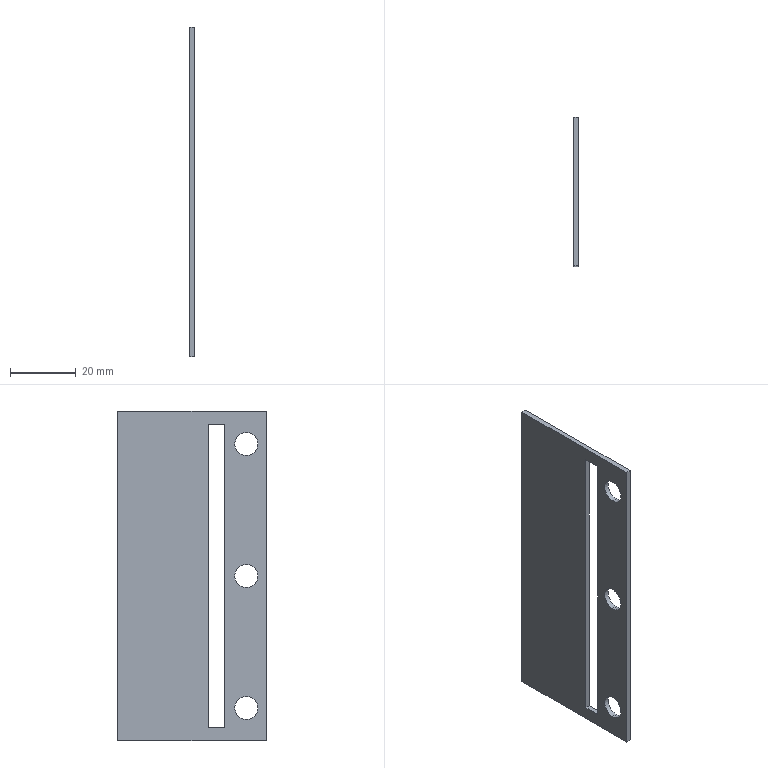Part | STEP file | SYL_0392D6J1SYL0380DJ100-207422 | 1 solid | 16 faces | box 1.5 x 45 x 100 mm | volume 5887 mm3 | plane 10 | cylinder 6 | commonest cylinder face diameters 7 x6
STEP:
#1=CARTESIAN_POINT('',(0.,6.,-3.5));
#2=VERTEX_POINT('',#1);
#3=CARTESIAN_POINT('',(0.,6.,3.5));
#4=VERTEX_POINT('',#3);
#5=CARTESIAN_POINT('',(0.,6.,0.));
#6=DIRECTION('',(1.,0.,0.));
#7=DIRECTION('',(0.,0.,-1.));
#8=AXIS2_PLACEMENT_3D('',#5,#6,#7);
#9=CIRCLE('',#8,3.5);
#10=EDGE_CURVE('',#2,#4,#9,.T.);
#11=ORIENTED_EDGE('',*,*,#10,.F.);
#12=CARTESIAN_POINT('',(1.5,6.,-3.5));
#13=VERTEX_POINT('',#12);
#14=CARTESIAN_POINT('',(1.5,6.,-3.5));
#15=DIRECTION('',(-1.,0.,0.));
#16=VECTOR('',#15,1000.);
#17=LINE('',#14,#16);
#18=EDGE_CURVE('',#13,#2,#17,.T.);
#19=ORIENTED_EDGE('',*,*,#18,.F.);
#20=CARTESIAN_POINT('',(1.5,6.,3.5));
#21=VERTEX_POINT('',#20);
#22=CARTESIAN_POINT('',(1.5,6.,0.));
#23=DIRECTION('',(-1.,0.,0.));
#24=DIRECTION('',(0.,0.,1.));
#25=AXIS2_PLACEMENT_3D('',#22,#23,#24);
#26=CIRCLE('',#25,3.5);
#27=EDGE_CURVE('',#21,#13,#26,.T.);
#28=ORIENTED_EDGE('',*,*,#27,.F.);
#29=CARTESIAN_POINT('',(1.5,6.,3.5));
#30=DIRECTION('',(-1.,0.,0.));
#31=VECTOR('',#30,1000.);
#32=LINE('',#29,#31);
#33=EDGE_CURVE('',#21,#4,#32,.T.);
#34=ORIENTED_EDGE('',*,*,#33,.T.);
#35=EDGE_LOOP('',(#11,#19,#28,#34));
#36=FACE_OUTER_BOUND('',#35,.T.);
#37=CARTESIAN_POINT('',(0.75,6.,0.));
#38=DIRECTION('',(1.,0.,0.));
#39=DIRECTION('',(0.,0.,-1.));
#40=AXIS2_PLACEMENT_3D('',#37,#38,#39);
#41=CYLINDRICAL_SURFACE('',#40,3.5);
#42=ADVANCED_FACE('',(#36),#41,.F.);
#43=ORIENTED_EDGE('',*,*,#33,.F.);
#44=CARTESIAN_POINT('',(1.5,6.,0.));
#45=DIRECTION('',(-1.,0.,0.));
#46=DIRECTION('',(0.,0.,-1.));
#47=AXIS2_PLACEMENT_3D('',#44,#45,#46);
#48=CIRCLE('',#47,3.5);
#49=EDGE_CURVE('',#13,#21,#48,.T.);
#50=ORIENTED_EDGE('',*,*,#49,.F.);
#51=ORIENTED_EDGE('',*,*,#18,.T.);
#52=CARTESIAN_POINT('',(0.,6.,0.));
#53=DIRECTION('',(1.,0.,0.));
#54=DIRECTION('',(0.,0.,1.));
#55=AXIS2_PLACEMENT_3D('',#52,#53,#54);
#56=CIRCLE('',#55,3.5);
#57=EDGE_CURVE('',#4,#2,#56,.T.);
#58=ORIENTED_EDGE('',*,*,#57,.F.);
#59=EDGE_LOOP('',(#43,#50,#51,#58));
#60=FACE_OUTER_BOUND('',#59,.T.);
#61=CARTESIAN_POINT('',(0.75,6.,0.));
#62=DIRECTION('',(1.,0.,0.));
#63=DIRECTION('',(0.,0.,-1.));
#64=AXIS2_PLACEMENT_3D('',#61,#62,#63);
#65=CYLINDRICAL_SURFACE('',#64,3.5);
#66=ADVANCED_FACE('',(#60),#65,.F.);
#67=CARTESIAN_POINT('',(0.,6.,-43.5));
#68=VERTEX_POINT('',#67);
#69=CARTESIAN_POINT('',(0.,6.,-36.5));
#70=VERTEX_POINT('',#69);
#71=CARTESIAN_POINT('',(0.,6.,-40.));
#72=DIRECTION('',(1.,0.,0.));
#73=DIRECTION('',(0.,0.,-1.));
#74=AXIS2_PLACEMENT_3D('',#71,#72,#73);
#75=CIRCLE('',#74,3.5);
#76=EDGE_CURVE('',#68,#70,#75,.T.);
#77=ORIENTED_EDGE('',*,*,#76,.F.);
#78=CARTESIAN_POINT('',(1.5,6.,-43.5));
#79=VERTEX_POINT('',#78);
#80=CARTESIAN_POINT('',(1.5,6.,-43.5));
#81=DIRECTION('',(-1.,0.,0.));
#82=VECTOR('',#81,1000.);
#83=LINE('',#80,#82);
#84=EDGE_CURVE('',#79,#68,#83,.T.);
#85=ORIENTED_EDGE('',*,*,#84,.F.);
#86=CARTESIAN_POINT('',(1.5,6.,-36.5));
#87=VERTEX_POINT('',#86);
#88=CARTESIAN_POINT('',(1.5,6.,-40.));
#89=DIRECTION('',(-1.,0.,0.));
#90=DIRECTION('',(0.,0.,1.));
#91=AXIS2_PLACEMENT_3D('',#88,#89,#90);
#92=CIRCLE('',#91,3.5);
#93=EDGE_CURVE('',#87,#79,#92,.T.);
#94=ORIENTED_EDGE('',*,*,#93,.F.);
#95=CARTESIAN_POINT('',(1.5,6.,-36.5));
#96=DIRECTION('',(-1.,0.,0.));
#97=VECTOR('',#96,1000.);
#98=LINE('',#95,#97);
#99=EDGE_CURVE('',#87,#70,#98,.T.);
#100=ORIENTED_EDGE('',*,*,#99,.T.);
#101=EDGE_LOOP('',(#77,#85,#94,#100));
#102=FACE_OUTER_BOUND('',#101,.T.);
#103=CARTESIAN_POINT('',(0.75,6.,-40.));
#104=DIRECTION('',(1.,0.,0.));
#105=DIRECTION('',(0.,0.,-1.));
#106=AXIS2_PLACEMENT_3D('',#103,#104,#105);
#107=CYLINDRICAL_SURFACE('',#106,3.5);
#108=ADVANCED_FACE('',(#102),#107,.F.);
#109=ORIENTED_EDGE('',*,*,#99,.F.);
#110=CARTESIAN_POINT('',(1.5,6.,-40.));
#111=DIRECTION('',(-1.,0.,0.));
#112=DIRECTION('',(0.,0.,-1.));
#113=AXIS2_PLACEMENT_3D('',#110,#111,#112);
#114=CIRCLE('',#113,3.5);
#115=EDGE_CURVE('',#79,#87,#114,.T.);
#116=ORIENTED_EDGE('',*,*,#115,.F.);
#117=ORIENTED_EDGE('',*,*,#84,.T.);
#118=CARTESIAN_POINT('',(0.,6.,-40.));
#119=DIRECTION('',(1.,0.,0.));
#120=DIRECTION('',(0.,0.,1.));
#121=AXIS2_PLACEMENT_3D('',#118,#119,#120);
#122=CIRCLE('',#121,3.5);
#123=EDGE_CURVE('',#70,#68,#122,.T.);
#124=ORIENTED_EDGE('',*,*,#123,.F.);
#125=EDGE_LOOP('',(#109,#116,#117,#124));
#126=FACE_OUTER_BOUND('',#125,.T.);
#127=CARTESIAN_POINT('',(0.75,6.,-40.));
#128=DIRECTION('',(1.,0.,0.));
#129=DIRECTION('',(0.,0.,-1.));
#130=AXIS2_PLACEMENT_3D('',#127,#128,#129);
#131=CYLINDRICAL_SURFACE('',#130,3.5);
#132=ADVANCED_FACE('',(#126),#131,.F.);
#133=CARTESIAN_POINT('',(0.,6.,36.5));
#134=VERTEX_POINT('',#133);
#135=CARTESIAN_POINT('',(0.,6.,43.5));
#136=VERTEX_POINT('',#135);
#137=CARTESIAN_POINT('',(0.,6.,40.));
#138=DIRECTION('',(1.,0.,0.));
#139=DIRECTION('',(0.,0.,-1.));
#140=AXIS2_PLACEMENT_3D('',#137,#138,#139);
#141=CIRCLE('',#140,3.5);
#142=EDGE_CURVE('',#134,#136,#141,.T.);
#143=ORIENTED_EDGE('',*,*,#142,.F.);
#144=CARTESIAN_POINT('',(1.5,6.,36.5));
#145=VERTEX_POINT('',#144);
#146=CARTESIAN_POINT('',(1.5,6.,36.5));
#147=DIRECTION('',(-1.,0.,0.));
#148=VECTOR('',#147,1000.);
#149=LINE('',#146,#148);
#150=EDGE_CURVE('',#145,#134,#149,.T.);
#151=ORIENTED_EDGE('',*,*,#150,.F.);
#152=CARTESIAN_POINT('',(1.5,6.,43.5));
#153=VERTEX_POINT('',#152);
#154=CARTESIAN_POINT('',(1.5,6.,40.));
#155=DIRECTION('',(-1.,0.,0.));
#156=DIRECTION('',(0.,0.,1.));
#157=AXIS2_PLACEMENT_3D('',#154,#155,#156);
#158=CIRCLE('',#157,3.5);
#159=EDGE_CURVE('',#153,#145,#158,.T.);
#160=ORIENTED_EDGE('',*,*,#159,.F.);
#161=CARTESIAN_POINT('',(1.5,6.,43.5));
#162=DIRECTION('',(-1.,0.,0.));
#163=VECTOR('',#162,1000.);
#164=LINE('',#161,#163);
#165=EDGE_CURVE('',#153,#136,#164,.T.);
#166=ORIENTED_EDGE('',*,*,#165,.T.);
#167=EDGE_LOOP('',(#143,#151,#160,#166));
#168=FACE_OUTER_BOUND('',#167,.T.);
#169=CARTESIAN_POINT('',(0.75,6.,40.));
#170=DIRECTION('',(1.,0.,0.));
#171=DIRECTION('',(0.,0.,-1.));
#172=AXIS2_PLACEMENT_3D('',#169,#170,#171);
#173=CYLINDRICAL_SURFACE('',#172,3.5);
#174=ADVANCED_FACE('',(#168),#173,.F.);
#175=ORIENTED_EDGE('',*,*,#165,.F.);
#176=CARTESIAN_POINT('',(1.5,6.,40.));
#177=DIRECTION('',(-1.,0.,0.));
#178=DIRECTION('',(0.,0.,-1.));
#179=AXIS2_PLACEMENT_3D('',#176,#177,#178);
#180=CIRCLE('',#179,3.5);
#181=EDGE_CURVE('',#145,#153,#180,.T.);
#182=ORIENTED_EDGE('',*,*,#181,.F.);
#183=ORIENTED_EDGE('',*,*,#150,.T.);
#184=CARTESIAN_POINT('',(0.,6.,40.));
#185=DIRECTION('',(1.,0.,0.));
#186=DIRECTION('',(0.,0.,1.));
#187=AXIS2_PLACEMENT_3D('',#184,#185,#186);
#188=CIRCLE('',#187,3.5);
#189=EDGE_CURVE('',#136,#134,#188,.T.);
#190=ORIENTED_EDGE('',*,*,#189,.F.);
#191=EDGE_LOOP('',(#175,#182,#183,#190));
#192=FACE_OUTER_BOUND('',#191,.T.);
#193=CARTESIAN_POINT('',(0.75,6.,40.));
#194=DIRECTION('',(1.,0.,0.));
#195=DIRECTION('',(0.,0.,-1.));
#196=AXIS2_PLACEMENT_3D('',#193,#194,#195);
#197=CYLINDRICAL_SURFACE('',#196,3.5);
#198=ADVANCED_FACE('',(#192),#197,.F.);
#199=CARTESIAN_POINT('',(0.,17.5,46.));
#200=VERTEX_POINT('',#199);
#201=CARTESIAN_POINT('',(1.5,17.5,46.));
#202=VERTEX_POINT('',#201);
#203=CARTESIAN_POINT('',(0.,17.5,46.));
#204=DIRECTION('',(1.,0.,0.));
#205=VECTOR('',#204,1000.);
#206=LINE('',#203,#205);
#207=EDGE_CURVE('',#200,#202,#206,.T.);
#208=ORIENTED_EDGE('',*,*,#207,.F.);
#209=CARTESIAN_POINT('',(0.,17.5,-46.));
#210=VERTEX_POINT('',#209);
#211=CARTESIAN_POINT('',(0.,17.5,-46.));
#212=DIRECTION('',(0.,0.,1.));
#213=VECTOR('',#212,1000.);
#214=LINE('',#211,#213);
#215=EDGE_CURVE('',#210,#200,#214,.T.);
#216=ORIENTED_EDGE('',*,*,#215,.F.);
#217=CARTESIAN_POINT('',(1.5,17.5,-46.));
#218=VERTEX_POINT('',#217);
#219=CARTESIAN_POINT('',(1.5,17.5,-46.));
#220=DIRECTION('',(-1.,0.,0.));
#221=VECTOR('',#220,1000.);
#222=LINE('',#219,#221);
#223=EDGE_CURVE('',#218,#210,#222,.T.);
#224=ORIENTED_EDGE('',*,*,#223,.F.);
#225=CARTESIAN_POINT('',(1.5,17.5,-46.));
#226=DIRECTION('',(0.,0.,1.));
#227=VECTOR('',#226,1000.);
#228=LINE('',#225,#227);
#229=EDGE_CURVE('',#218,#202,#228,.T.);
#230=ORIENTED_EDGE('',*,*,#229,.T.);
#231=EDGE_LOOP('',(#208,#216,#224,#230));
#232=FACE_OUTER_BOUND('',#231,.T.);
#233=CARTESIAN_POINT('',(0.75,17.5,0.));
#234=DIRECTION('',(0.,1.,0.));
#235=DIRECTION('',(1.,0.,0.));
#236=AXIS2_PLACEMENT_3D('',#233,#234,#235);
#237=PLANE('',#236);
#238=ADVANCED_FACE('',(#232),#237,.F.);
#239=CARTESIAN_POINT('',(1.5,12.5,46.));
#240=VERTEX_POINT('',#239);
#241=CARTESIAN_POINT('',(0.,12.5,46.));
#242=VERTEX_POINT('',#241);
#243=CARTESIAN_POINT('',(1.5,12.5,46.));
#244=DIRECTION('',(-1.,0.,0.));
#245=VECTOR('',#244,1000.);
#246=LINE('',#243,#245);
#247=EDGE_CURVE('',#240,#242,#246,.T.);
#248=ORIENTED_EDGE('',*,*,#247,.T.);
#249=CARTESIAN_POINT('',(0.,17.5,46.));
#250=DIRECTION('',(0.,-1.,0.));
#251=VECTOR('',#250,1000.);
#252=LINE('',#249,#251);
#253=EDGE_CURVE('',#200,#242,#252,.T.);
#254=ORIENTED_EDGE('',*,*,#253,.F.);
#255=ORIENTED_EDGE('',*,*,#207,.T.);
#256=CARTESIAN_POINT('',(1.5,17.5,46.));
#257=DIRECTION('',(0.,-1.,0.));
#258=VECTOR('',#257,1000.);
#259=LINE('',#256,#258);
#260=EDGE_CURVE('',#202,#240,#259,.T.);
#261=ORIENTED_EDGE('',*,*,#260,.T.);
#262=EDGE_LOOP('',(#248,#254,#255,#261));
#263=FACE_OUTER_BOUND('',#262,.T.);
#264=CARTESIAN_POINT('',(0.75,15.,46.));
#265=DIRECTION('',(0.,0.,1.));
#266=DIRECTION('',(1.,0.,0.));
#267=AXIS2_PLACEMENT_3D('',#264,#265,#266);
#268=PLANE('',#267);
#269=ADVANCED_FACE('',(#263),#268,.F.);
#270=CARTESIAN_POINT('',(1.5,12.5,-46.));
#271=VERTEX_POINT('',#270);
#272=CARTESIAN_POINT('',(0.,12.5,-46.));
#273=VERTEX_POINT('',#272);
#274=CARTESIAN_POINT('',(1.5,12.5,-46.));
#275=DIRECTION('',(-1.,0.,0.));
#276=VECTOR('',#275,1000.);
#277=LINE('',#274,#276);
#278=EDGE_CURVE('',#271,#273,#277,.T.);
#279=ORIENTED_EDGE('',*,*,#278,.T.);
#280=CARTESIAN_POINT('',(0.,12.5,46.));
#281=DIRECTION('',(0.,0.,-1.));
#282=VECTOR('',#281,1000.);
#283=LINE('',#280,#282);
#284=EDGE_CURVE('',#242,#273,#283,.T.);
#285=ORIENTED_EDGE('',*,*,#284,.F.);
#286=ORIENTED_EDGE('',*,*,#247,.F.);
#287=CARTESIAN_POINT('',(1.5,12.5,46.));
#288=DIRECTION('',(0.,0.,-1.));
#289=VECTOR('',#288,1000.);
#290=LINE('',#287,#289);
#291=EDGE_CURVE('',#240,#271,#290,.T.);
#292=ORIENTED_EDGE('',*,*,#291,.T.);
#293=EDGE_LOOP('',(#279,#285,#286,#292));
#294=FACE_OUTER_BOUND('',#293,.T.);
#295=CARTESIAN_POINT('',(0.75,12.5,0.));
#296=DIRECTION('',(0.,-1.,0.));
#297=DIRECTION('',(0.,0.,-1.));
#298=AXIS2_PLACEMENT_3D('',#295,#296,#297);
#299=PLANE('',#298);
#300=ADVANCED_FACE('',(#294),#299,.F.);
#301=ORIENTED_EDGE('',*,*,#10,.T.);
#302=ORIENTED_EDGE('',*,*,#57,.T.);
#303=EDGE_LOOP('',(#301,#302));
#304=FACE_BOUND('',#303,.T.);
#305=ORIENTED_EDGE('',*,*,#76,.T.);
#306=ORIENTED_EDGE('',*,*,#123,.T.);
#307=EDGE_LOOP('',(#305,#306));
#308=FACE_BOUND('',#307,.T.);
#309=ORIENTED_EDGE('',*,*,#142,.T.);
#310=ORIENTED_EDGE('',*,*,#189,.T.);
#311=EDGE_LOOP('',(#309,#310));
#312=FACE_BOUND('',#311,.T.);
#313=CARTESIAN_POINT('',(0.,12.5,-46.));
#314=DIRECTION('',(0.,1.,0.));
#315=VECTOR('',#314,1000.);
#316=LINE('',#313,#315);
#317=EDGE_CURVE('',#273,#210,#316,.T.);
#318=ORIENTED_EDGE('',*,*,#317,.T.);
#319=ORIENTED_EDGE('',*,*,#215,.T.);
#320=ORIENTED_EDGE('',*,*,#253,.T.);
#321=ORIENTED_EDGE('',*,*,#284,.T.);
#322=EDGE_LOOP('',(#318,#319,#320,#321));
#323=FACE_BOUND('',#322,.T.);
#324=CARTESIAN_POINT('',(0.,0.,-50.));
#325=VERTEX_POINT('',#324);
#326=CARTESIAN_POINT('',(0.,0.,50.));
#327=VERTEX_POINT('',#326);
#328=CARTESIAN_POINT('',(0.,0.,-50.));
#329=DIRECTION('',(0.,0.,1.));
#330=VECTOR('',#329,1000.);
#331=LINE('',#328,#330);
#332=EDGE_CURVE('',#325,#327,#331,.T.);
#333=ORIENTED_EDGE('',*,*,#332,.T.);
#334=CARTESIAN_POINT('',(0.,45.,50.));
#335=VERTEX_POINT('',#334);
#336=CARTESIAN_POINT('',(0.,0.,50.));
#337=DIRECTION('',(0.,1.,0.));
#338=VECTOR('',#337,1000.);
#339=LINE('',#336,#338);
#340=EDGE_CURVE('',#327,#335,#339,.T.);
#341=ORIENTED_EDGE('',*,*,#340,.T.);
#342=CARTESIAN_POINT('',(0.,45.,-50.));
#343=VERTEX_POINT('',#342);
#344=CARTESIAN_POINT('',(0.,45.,50.));
#345=DIRECTION('',(0.,0.,-1.));
#346=VECTOR('',#345,1000.);
#347=LINE('',#344,#346);
#348=EDGE_CURVE('',#335,#343,#347,.T.);
#349=ORIENTED_EDGE('',*,*,#348,.T.);
#350=CARTESIAN_POINT('',(0.,45.,-50.));
#351=DIRECTION('',(0.,-1.,0.));
#352=VECTOR('',#351,1000.);
#353=LINE('',#350,#352);
#354=EDGE_CURVE('',#343,#325,#353,.T.);
#355=ORIENTED_EDGE('',*,*,#354,.T.);
#356=EDGE_LOOP('',(#333,#341,#349,#355));
#357=FACE_OUTER_BOUND('',#356,.T.);
#358=CARTESIAN_POINT('',(0.,0.,0.));
#359=DIRECTION('',(1.,0.,0.));
#360=DIRECTION('',(0.,1.,0.));
#361=AXIS2_PLACEMENT_3D('',#358,#359,#360);
#362=PLANE('',#361);
#363=ADVANCED_FACE('',(#304,#308,#312,#323,#357),#362,.F.);
#364=CARTESIAN_POINT('',(1.5,0.,-50.));
#365=VERTEX_POINT('',#364);
#366=CARTESIAN_POINT('',(1.5,0.,-50.));
#367=DIRECTION('',(-1.,0.,0.));
#368=VECTOR('',#367,1000.);
#369=LINE('',#366,#368);
#370=EDGE_CURVE('',#365,#325,#369,.T.);
#371=ORIENTED_EDGE('',*,*,#370,.T.);
#372=ORIENTED_EDGE('',*,*,#354,.F.);
#373=CARTESIAN_POINT('',(1.5,45.,-50.));
#374=VERTEX_POINT('',#373);
#375=CARTESIAN_POINT('',(1.5,45.,-50.));
#376=DIRECTION('',(-1.,0.,0.));
#377=VECTOR('',#376,1000.);
#378=LINE('',#375,#377);
#379=EDGE_CURVE('',#374,#343,#378,.T.);
#380=ORIENTED_EDGE('',*,*,#379,.F.);
#381=CARTESIAN_POINT('',(1.5,45.,-50.));
#382=DIRECTION('',(0.,-1.,0.));
#383=VECTOR('',#382,1000.);
#384=LINE('',#381,#383);
#385=EDGE_CURVE('',#374,#365,#384,.T.);
#386=ORIENTED_EDGE('',*,*,#385,.T.);
#387=EDGE_LOOP('',(#371,#372,#380,#386));
#388=FACE_OUTER_BOUND('',#387,.T.);
#389=CARTESIAN_POINT('',(0.75,22.5,-50.));
#390=DIRECTION('',(0.,0.,1.));
#391=DIRECTION('',(1.,0.,0.));
#392=AXIS2_PLACEMENT_3D('',#389,#390,#391);
#393=PLANE('',#392);
#394=ADVANCED_FACE('',(#388),#393,.F.);
#395=CARTESIAN_POINT('',(1.5,0.,50.));
#396=VERTEX_POINT('',#395);
#397=CARTESIAN_POINT('',(1.5,0.,50.));
#398=DIRECTION('',(-1.,0.,0.));
#399=VECTOR('',#398,1000.);
#400=LINE('',#397,#399);
#401=EDGE_CURVE('',#396,#327,#400,.T.);
#402=ORIENTED_EDGE('',*,*,#401,.T.);
#403=ORIENTED_EDGE('',*,*,#332,.F.);
#404=ORIENTED_EDGE('',*,*,#370,.F.);
#405=CARTESIAN_POINT('',(1.5,0.,-50.));
#406=DIRECTION('',(0.,0.,1.));
#407=VECTOR('',#406,1000.);
#408=LINE('',#405,#407);
#409=EDGE_CURVE('',#365,#396,#408,.T.);
#410=ORIENTED_EDGE('',*,*,#409,.T.);
#411=EDGE_LOOP('',(#402,#403,#404,#410));
#412=FACE_OUTER_BOUND('',#411,.T.);
#413=CARTESIAN_POINT('',(0.75,0.,0.));
#414=DIRECTION('',(0.,1.,0.));
#415=DIRECTION('',(1.,0.,0.));
#416=AXIS2_PLACEMENT_3D('',#413,#414,#415);
#417=PLANE('',#416);
#418=ADVANCED_FACE('',(#412),#417,.F.);
#419=CARTESIAN_POINT('',(1.5,45.,50.));
#420=VERTEX_POINT('',#419);
#421=CARTESIAN_POINT('',(0.,45.,50.));
#422=DIRECTION('',(1.,0.,0.));
#423=VECTOR('',#422,1000.);
#424=LINE('',#421,#423);
#425=EDGE_CURVE('',#335,#420,#424,.T.);
#426=ORIENTED_EDGE('',*,*,#425,.F.);
#427=ORIENTED_EDGE('',*,*,#340,.F.);
#428=ORIENTED_EDGE('',*,*,#401,.F.);
#429=CARTESIAN_POINT('',(1.5,0.,50.));
#430=DIRECTION('',(0.,1.,0.));
#431=VECTOR('',#430,1000.);
#432=LINE('',#429,#431);
#433=EDGE_CURVE('',#396,#420,#432,.T.);
#434=ORIENTED_EDGE('',*,*,#433,.T.);
#435=EDGE_LOOP('',(#426,#427,#428,#434));
#436=FACE_OUTER_BOUND('',#435,.T.);
#437=CARTESIAN_POINT('',(0.75,22.5,50.));
#438=DIRECTION('',(0.,0.,-1.));
#439=DIRECTION('',(0.,-1.,0.));
#440=AXIS2_PLACEMENT_3D('',#437,#438,#439);
#441=PLANE('',#440);
#442=ADVANCED_FACE('',(#436),#441,.F.);
#443=ORIENTED_EDGE('',*,*,#379,.T.);
#444=ORIENTED_EDGE('',*,*,#348,.F.);
#445=ORIENTED_EDGE('',*,*,#425,.T.);
#446=CARTESIAN_POINT('',(1.5,45.,50.));
#447=DIRECTION('',(0.,0.,-1.));
#448=VECTOR('',#447,1000.);
#449=LINE('',#446,#448);
#450=EDGE_CURVE('',#420,#374,#449,.T.);
#451=ORIENTED_EDGE('',*,*,#450,.T.);
#452=EDGE_LOOP('',(#443,#444,#445,#451));
#453=FACE_OUTER_BOUND('',#452,.T.);
#454=CARTESIAN_POINT('',(0.75,45.,0.));
#455=DIRECTION('',(0.,-1.,0.));
#456=DIRECTION('',(0.,0.,-1.));
#457=AXIS2_PLACEMENT_3D('',#454,#455,#456);
#458=PLANE('',#457);
#459=ADVANCED_FACE('',(#453),#458,.F.);
#460=ORIENTED_EDGE('',*,*,#159,.T.);
#461=ORIENTED_EDGE('',*,*,#181,.T.);
#462=EDGE_LOOP('',(#460,#461));
#463=FACE_BOUND('',#462,.T.);
#464=ORIENTED_EDGE('',*,*,#93,.T.);
#465=ORIENTED_EDGE('',*,*,#115,.T.);
#466=EDGE_LOOP('',(#464,#465));
#467=FACE_BOUND('',#466,.T.);
#468=ORIENTED_EDGE('',*,*,#27,.T.);
#469=ORIENTED_EDGE('',*,*,#49,.T.);
#470=EDGE_LOOP('',(#468,#469));
#471=FACE_BOUND('',#470,.T.);
#472=ORIENTED_EDGE('',*,*,#229,.F.);
#473=CARTESIAN_POINT('',(1.5,12.5,-46.));
#474=DIRECTION('',(0.,1.,0.));
#475=VECTOR('',#474,1000.);
#476=LINE('',#473,#475);
#477=EDGE_CURVE('',#271,#218,#476,.T.);
#478=ORIENTED_EDGE('',*,*,#477,.F.);
#479=ORIENTED_EDGE('',*,*,#291,.F.);
#480=ORIENTED_EDGE('',*,*,#260,.F.);
#481=EDGE_LOOP('',(#472,#478,#479,#480));
#482=FACE_BOUND('',#481,.T.);
#483=ORIENTED_EDGE('',*,*,#433,.F.);
#484=ORIENTED_EDGE('',*,*,#409,.F.);
#485=ORIENTED_EDGE('',*,*,#385,.F.);
#486=ORIENTED_EDGE('',*,*,#450,.F.);
#487=EDGE_LOOP('',(#483,#484,#485,#486));
#488=FACE_OUTER_BOUND('',#487,.T.);
#489=CARTESIAN_POINT('',(1.5,0.,0.));
#490=DIRECTION('',(1.,0.,0.));
#491=DIRECTION('',(0.,1.,0.));
#492=AXIS2_PLACEMENT_3D('',#489,#490,#491);
#493=PLANE('',#492);
#494=ADVANCED_FACE('',(#463,#467,#471,#482,#488),#493,.T.);
#495=ORIENTED_EDGE('',*,*,#223,.T.);
#496=ORIENTED_EDGE('',*,*,#317,.F.);
#497=ORIENTED_EDGE('',*,*,#278,.F.);
#498=ORIENTED_EDGE('',*,*,#477,.T.);
#499=EDGE_LOOP('',(#495,#496,#497,#498));
#500=FACE_OUTER_BOUND('',#499,.T.);
#501=CARTESIAN_POINT('',(0.75,15.,-46.));
#502=DIRECTION('',(0.,0.,-1.));
#503=DIRECTION('',(0.,-1.,0.));
#504=AXIS2_PLACEMENT_3D('',#501,#502,#503);
#505=PLANE('',#504);
#506=ADVANCED_FACE('',(#500),#505,.F.);
#507=CLOSED_SHELL('',(#42,#66,#108,#132,#174,#198,#238,#269,#300,#363,#394,#418,#442,#459,#494,#506));
#508=MANIFOLD_SOLID_BREP('',#507);
#509=CARTESIAN_POINT('',(0.,0.,0.));
#510=DIRECTION('',(0.,0.,1.));
#511=DIRECTION('',(1.,0.,0.));
#512=AXIS2_PLACEMENT_3D('',#509,#510,#511);
#513=(LENGTH_UNIT()NAMED_UNIT(*)SI_UNIT(.MILLI.,.METRE.));
#514=UNCERTAINTY_MEASURE_WITH_UNIT(LENGTH_MEASURE(0.00001),#513,'','');
#515=(NAMED_UNIT(*)PLANE_ANGLE_UNIT()SI_UNIT($,.RADIAN.));
#516=(NAMED_UNIT(*)SI_UNIT($,.STERADIAN.)SOLID_ANGLE_UNIT());
#517=(GEOMETRIC_REPRESENTATION_CONTEXT(3)GLOBAL_UNCERTAINTY_ASSIGNED_CONTEXT((#514))GLOBAL_UNIT_ASSIGNED_CONTEXT((#513,#515,#516))REPRESENTATION_CONTEXT('',''));
#518=ADVANCED_BREP_SHAPE_REPRESENTATION('',(#508,#512),#517);